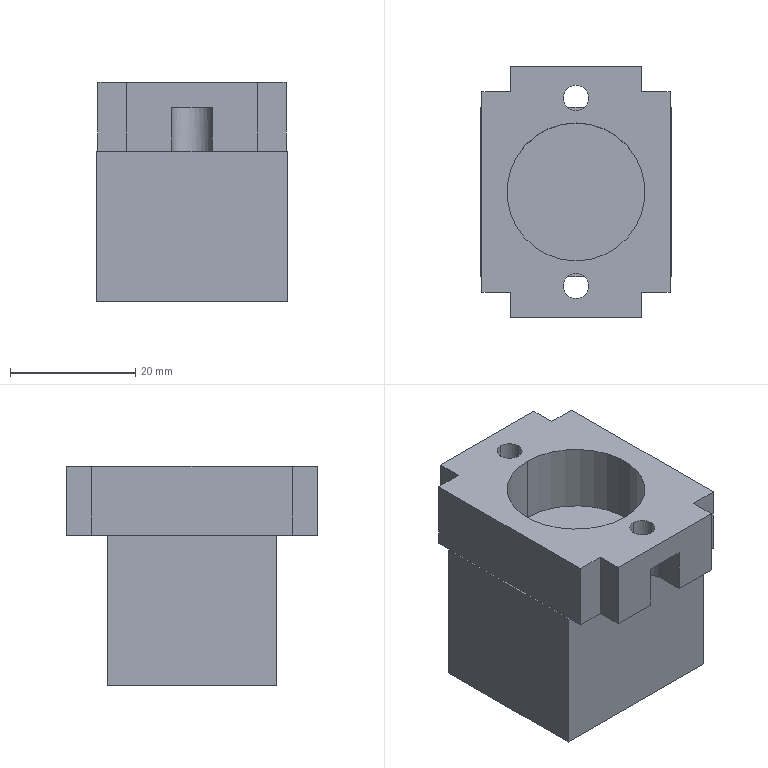Part | SolidWorks | features ImportedCurve 15, BaseBody 1 | 1 solid | 41 faces | box 30.5 x 40 x 35 mm | volume 27294 mm3 | plane 33 | cylinder 8 | commonest cylinder face diameters 4 x4 6.5 x2 22 x2
STEP:
#1=CARTESIAN_POINT('',(3.25,16.,0.));
#2=VERTEX_POINT('',#1);
#3=CARTESIAN_POINT('',(3.25,16.,7.));
#4=VERTEX_POINT('',#3);
#5=CARTESIAN_POINT('',(3.25,16.,0.));
#6=DIRECTION('',(0.,0.,1.));
#7=VECTOR('',#6,1000.);
#8=LINE('',#5,#7);
#9=EDGE_CURVE('',#2,#4,#8,.T.);
#10=ORIENTED_EDGE('',*,*,#9,.T.);
#11=CARTESIAN_POINT('',(3.25,20.,7.));
#12=VERTEX_POINT('',#11);
#13=CARTESIAN_POINT('',(3.25,20.,7.));
#14=DIRECTION('',(0.,-1.,0.));
#15=VECTOR('',#14,1000.);
#16=LINE('',#13,#15);
#17=EDGE_CURVE('',#12,#4,#16,.T.);
#18=ORIENTED_EDGE('',*,*,#17,.F.);
#19=CARTESIAN_POINT('',(3.25,20.,0.));
#20=VERTEX_POINT('',#19);
#21=CARTESIAN_POINT('',(3.25,20.,0.));
#22=DIRECTION('',(0.,0.,1.));
#23=VECTOR('',#22,1000.);
#24=LINE('',#21,#23);
#25=EDGE_CURVE('',#20,#12,#24,.T.);
#26=ORIENTED_EDGE('',*,*,#25,.F.);
#27=CARTESIAN_POINT('',(3.25,20.,0.));
#28=DIRECTION('',(0.,-1.,0.));
#29=VECTOR('',#28,1000.);
#30=LINE('',#27,#29);
#31=EDGE_CURVE('',#20,#2,#30,.T.);
#32=ORIENTED_EDGE('',*,*,#31,.T.);
#33=EDGE_LOOP('',(#10,#18,#26,#32));
#34=FACE_OUTER_BOUND('',#33,.T.);
#35=CARTESIAN_POINT('',(3.25,20.,0.));
#36=DIRECTION('',(1.,0.,0.));
#37=DIRECTION('',(0.,-1.,0.));
#38=AXIS2_PLACEMENT_3D('',#35,#36,#37);
#39=PLANE('',#38);
#40=ADVANCED_FACE('',(#34),#39,.F.);
#41=CARTESIAN_POINT('',(-15.25,13.5,0.));
#42=VERTEX_POINT('',#41);
#43=CARTESIAN_POINT('',(-15.25,13.5,-24.));
#44=VERTEX_POINT('',#43);
#45=CARTESIAN_POINT('',(-15.25,13.5,0.));
#46=DIRECTION('',(0.,0.,-1.));
#47=VECTOR('',#46,1000.);
#48=LINE('',#45,#47);
#49=EDGE_CURVE('',#42,#44,#48,.T.);
#50=ORIENTED_EDGE('',*,*,#49,.T.);
#51=CARTESIAN_POINT('',(-15.25,-13.5,-24.));
#52=VERTEX_POINT('',#51);
#53=CARTESIAN_POINT('',(-15.25,-13.5,-24.));
#54=DIRECTION('',(0.,1.,0.));
#55=VECTOR('',#54,1000.);
#56=LINE('',#53,#55);
#57=EDGE_CURVE('',#52,#44,#56,.T.);
#58=ORIENTED_EDGE('',*,*,#57,.F.);
#59=CARTESIAN_POINT('',(-15.25,-13.5,0.));
#60=VERTEX_POINT('',#59);
#61=CARTESIAN_POINT('',(-15.25,-13.5,0.));
#62=DIRECTION('',(0.,0.,-1.));
#63=VECTOR('',#62,1000.);
#64=LINE('',#61,#63);
#65=EDGE_CURVE('',#60,#52,#64,.T.);
#66=ORIENTED_EDGE('',*,*,#65,.F.);
#67=CARTESIAN_POINT('',(-15.25,-13.5,0.));
#68=DIRECTION('',(0.,1.,0.));
#69=VECTOR('',#68,1000.);
#70=LINE('',#67,#69);
#71=EDGE_CURVE('',#60,#42,#70,.T.);
#72=ORIENTED_EDGE('',*,*,#71,.T.);
#73=EDGE_LOOP('',(#50,#58,#66,#72));
#74=FACE_OUTER_BOUND('',#73,.T.);
#75=CARTESIAN_POINT('',(-15.25,-13.5,0.));
#76=DIRECTION('',(-1.,0.,0.));
#77=DIRECTION('',(0.,1.,0.));
#78=AXIS2_PLACEMENT_3D('',#75,#76,#77);
#79=PLANE('',#78);
#80=ADVANCED_FACE('',(#74),#79,.T.);
#81=CARTESIAN_POINT('',(15.25,13.5,-24.));
#82=VERTEX_POINT('',#81);
#83=CARTESIAN_POINT('',(-15.25,13.5,-24.));
#84=DIRECTION('',(1.,0.,0.));
#85=VECTOR('',#84,1000.);
#86=LINE('',#83,#85);
#87=EDGE_CURVE('',#44,#82,#86,.T.);
#88=ORIENTED_EDGE('',*,*,#87,.T.);
#89=CARTESIAN_POINT('',(15.25,-13.5,-24.));
#90=VERTEX_POINT('',#89);
#91=CARTESIAN_POINT('',(15.25,13.5,-24.));
#92=DIRECTION('',(0.,-1.,0.));
#93=VECTOR('',#92,1000.);
#94=LINE('',#91,#93);
#95=EDGE_CURVE('',#82,#90,#94,.T.);
#96=ORIENTED_EDGE('',*,*,#95,.T.);
#97=CARTESIAN_POINT('',(15.25,-13.5,-24.));
#98=DIRECTION('',(-1.,0.,0.));
#99=VECTOR('',#98,1000.);
#100=LINE('',#97,#99);
#101=EDGE_CURVE('',#90,#52,#100,.T.);
#102=ORIENTED_EDGE('',*,*,#101,.T.);
#103=ORIENTED_EDGE('',*,*,#57,.T.);
#104=EDGE_LOOP('',(#88,#96,#102,#103));
#105=FACE_OUTER_BOUND('',#104,.T.);
#106=CARTESIAN_POINT('',(0.,0.,-24.));
#107=DIRECTION('',(0.,0.,-1.));
#108=DIRECTION('',(1.,0.,0.));
#109=AXIS2_PLACEMENT_3D('',#106,#107,#108);
#110=PLANE('',#109);
#111=ADVANCED_FACE('',(#105),#110,.T.);
#112=CARTESIAN_POINT('',(15.25,-13.5,0.));
#113=VERTEX_POINT('',#112);
#114=CARTESIAN_POINT('',(15.25,-13.5,0.));
#115=DIRECTION('',(0.,0.,-1.));
#116=VECTOR('',#115,1000.);
#117=LINE('',#114,#116);
#118=EDGE_CURVE('',#113,#90,#117,.T.);
#119=ORIENTED_EDGE('',*,*,#118,.T.);
#120=ORIENTED_EDGE('',*,*,#95,.F.);
#121=CARTESIAN_POINT('',(15.25,13.5,0.));
#122=VERTEX_POINT('',#121);
#123=CARTESIAN_POINT('',(15.25,13.5,0.));
#124=DIRECTION('',(0.,0.,-1.));
#125=VECTOR('',#124,1000.);
#126=LINE('',#123,#125);
#127=EDGE_CURVE('',#122,#82,#126,.T.);
#128=ORIENTED_EDGE('',*,*,#127,.F.);
#129=CARTESIAN_POINT('',(15.25,13.5,0.));
#130=DIRECTION('',(0.,-1.,0.));
#131=VECTOR('',#130,1000.);
#132=LINE('',#129,#131);
#133=EDGE_CURVE('',#122,#113,#132,.T.);
#134=ORIENTED_EDGE('',*,*,#133,.T.);
#135=EDGE_LOOP('',(#119,#120,#128,#134));
#136=FACE_OUTER_BOUND('',#135,.T.);
#137=CARTESIAN_POINT('',(15.25,13.5,0.));
#138=DIRECTION('',(1.,0.,0.));
#139=DIRECTION('',(0.,-1.,0.));
#140=AXIS2_PLACEMENT_3D('',#137,#138,#139);
#141=PLANE('',#140);
#142=ADVANCED_FACE('',(#136),#141,.T.);
#143=ORIENTED_EDGE('',*,*,#133,.F.);
#144=CARTESIAN_POINT('',(15.,13.5,0.));
#145=VERTEX_POINT('',#144);
#146=CARTESIAN_POINT('',(15.,13.5,0.));
#147=DIRECTION('',(1.,0.,0.));
#148=VECTOR('',#147,1000.);
#149=LINE('',#146,#148);
#150=EDGE_CURVE('',#145,#122,#149,.T.);
#151=ORIENTED_EDGE('',*,*,#150,.F.);
#152=CARTESIAN_POINT('',(15.,-13.5,0.));
#153=VERTEX_POINT('',#152);
#154=CARTESIAN_POINT('',(15.,13.5,0.));
#155=DIRECTION('',(0.,-1.,0.));
#156=VECTOR('',#155,1000.);
#157=LINE('',#154,#156);
#158=EDGE_CURVE('',#145,#153,#157,.T.);
#159=ORIENTED_EDGE('',*,*,#158,.T.);
#160=CARTESIAN_POINT('',(15.25,-13.5,0.));
#161=DIRECTION('',(-1.,0.,0.));
#162=VECTOR('',#161,1000.);
#163=LINE('',#160,#162);
#164=EDGE_CURVE('',#113,#153,#163,.T.);
#165=ORIENTED_EDGE('',*,*,#164,.F.);
#166=EDGE_LOOP('',(#143,#151,#159,#165));
#167=FACE_OUTER_BOUND('',#166,.T.);
#168=CARTESIAN_POINT('',(0.,0.,0.));
#169=DIRECTION('',(0.,0.,-1.));
#170=DIRECTION('',(1.,0.,0.));
#171=AXIS2_PLACEMENT_3D('',#168,#169,#170);
#172=PLANE('',#171);
#173=ADVANCED_FACE('',(#167),#172,.F.);
#174=CARTESIAN_POINT('',(0.,-11.,11.));
#175=VERTEX_POINT('',#174);
#176=CARTESIAN_POINT('',(0.,-11.,0.));
#177=VERTEX_POINT('',#176);
#178=CARTESIAN_POINT('',(0.,-11.,11.));
#179=DIRECTION('',(0.,0.,-1.));
#180=VECTOR('',#179,1000.);
#181=LINE('',#178,#180);
#182=EDGE_CURVE('',#175,#177,#181,.T.);
#183=ORIENTED_EDGE('',*,*,#182,.F.);
#184=CARTESIAN_POINT('',(0.,11.,11.));
#185=VERTEX_POINT('',#184);
#186=CARTESIAN_POINT('',(0.,0.,11.));
#187=DIRECTION('',(0.,0.,1.));
#188=DIRECTION('',(0.,-1.,0.));
#189=AXIS2_PLACEMENT_3D('',#186,#187,#188);
#190=CIRCLE('',#189,11.);
#191=EDGE_CURVE('',#175,#185,#190,.T.);
#192=ORIENTED_EDGE('',*,*,#191,.T.);
#193=CARTESIAN_POINT('',(0.,11.,0.));
#194=VERTEX_POINT('',#193);
#195=CARTESIAN_POINT('',(0.,11.,11.));
#196=DIRECTION('',(0.,0.,-1.));
#197=VECTOR('',#196,1000.);
#198=LINE('',#195,#197);
#199=EDGE_CURVE('',#185,#194,#198,.T.);
#200=ORIENTED_EDGE('',*,*,#199,.T.);
#201=CARTESIAN_POINT('',(0.,0.,0.));
#202=DIRECTION('',(0.,0.,1.));
#203=DIRECTION('',(0.,-1.,0.));
#204=AXIS2_PLACEMENT_3D('',#201,#202,#203);
#205=CIRCLE('',#204,11.);
#206=EDGE_CURVE('',#177,#194,#205,.T.);
#207=ORIENTED_EDGE('',*,*,#206,.F.);
#208=EDGE_LOOP('',(#183,#192,#200,#207));
#209=FACE_OUTER_BOUND('',#208,.T.);
#210=CARTESIAN_POINT('',(0.,0.,11.));
#211=DIRECTION('',(0.,0.,1.));
#212=DIRECTION('',(0.,1.,0.));
#213=AXIS2_PLACEMENT_3D('',#210,#211,#212);
#214=CYLINDRICAL_SURFACE('',#213,11.);
#215=ADVANCED_FACE('',(#209),#214,.F.);
#216=ORIENTED_EDGE('',*,*,#206,.T.);
#217=CARTESIAN_POINT('',(0.,0.,0.));
#218=DIRECTION('',(0.,0.,1.));
#219=DIRECTION('',(0.,1.,0.));
#220=AXIS2_PLACEMENT_3D('',#217,#218,#219);
#221=CIRCLE('',#220,11.);
#222=EDGE_CURVE('',#194,#177,#221,.T.);
#223=ORIENTED_EDGE('',*,*,#222,.T.);
#224=EDGE_LOOP('',(#216,#223));
#225=FACE_OUTER_BOUND('',#224,.T.);
#226=CARTESIAN_POINT('',(0.,0.,0.));
#227=DIRECTION('',(0.,0.,-1.));
#228=DIRECTION('',(1.,0.,0.));
#229=AXIS2_PLACEMENT_3D('',#226,#227,#228);
#230=PLANE('',#229);
#231=ADVANCED_FACE('',(#225),#230,.F.);
#232=ORIENTED_EDGE('',*,*,#199,.F.);
#233=CARTESIAN_POINT('',(0.,0.,11.));
#234=DIRECTION('',(0.,0.,1.));
#235=DIRECTION('',(0.,1.,0.));
#236=AXIS2_PLACEMENT_3D('',#233,#234,#235);
#237=CIRCLE('',#236,11.);
#238=EDGE_CURVE('',#185,#175,#237,.T.);
#239=ORIENTED_EDGE('',*,*,#238,.T.);
#240=ORIENTED_EDGE('',*,*,#182,.T.);
#241=ORIENTED_EDGE('',*,*,#222,.F.);
#242=EDGE_LOOP('',(#232,#239,#240,#241));
#243=FACE_OUTER_BOUND('',#242,.T.);
#244=CARTESIAN_POINT('',(0.,0.,11.));
#245=DIRECTION('',(0.,0.,1.));
#246=DIRECTION('',(0.,1.,0.));
#247=AXIS2_PLACEMENT_3D('',#244,#245,#246);
#248=CYLINDRICAL_SURFACE('',#247,11.);
#249=ADVANCED_FACE('',(#243),#248,.F.);
#250=CARTESIAN_POINT('',(0.,17.,11.));
#251=VERTEX_POINT('',#250);
#252=CARTESIAN_POINT('',(0.,17.,7.));
#253=VERTEX_POINT('',#252);
#254=CARTESIAN_POINT('',(0.,17.,11.));
#255=DIRECTION('',(0.,0.,-1.));
#256=VECTOR('',#255,1000.);
#257=LINE('',#254,#256);
#258=EDGE_CURVE('',#251,#253,#257,.T.);
#259=ORIENTED_EDGE('',*,*,#258,.T.);
#260=CARTESIAN_POINT('',(0.,13.,7.));
#261=VERTEX_POINT('',#260);
#262=CARTESIAN_POINT('',(0.,15.,7.));
#263=DIRECTION('',(0.,0.,1.));
#264=DIRECTION('',(0.,-1.,0.));
#265=AXIS2_PLACEMENT_3D('',#262,#263,#264);
#266=CIRCLE('',#265,2.);
#267=EDGE_CURVE('',#261,#253,#266,.T.);
#268=ORIENTED_EDGE('',*,*,#267,.F.);
#269=CARTESIAN_POINT('',(0.,13.,11.));
#270=VERTEX_POINT('',#269);
#271=CARTESIAN_POINT('',(0.,13.,11.));
#272=DIRECTION('',(0.,0.,-1.));
#273=VECTOR('',#272,1000.);
#274=LINE('',#271,#273);
#275=EDGE_CURVE('',#270,#261,#274,.T.);
#276=ORIENTED_EDGE('',*,*,#275,.F.);
#277=CARTESIAN_POINT('',(0.,15.,11.));
#278=DIRECTION('',(0.,0.,1.));
#279=DIRECTION('',(0.,-1.,0.));
#280=AXIS2_PLACEMENT_3D('',#277,#278,#279);
#281=CIRCLE('',#280,2.);
#282=EDGE_CURVE('',#270,#251,#281,.T.);
#283=ORIENTED_EDGE('',*,*,#282,.T.);
#284=EDGE_LOOP('',(#259,#268,#276,#283));
#285=FACE_OUTER_BOUND('',#284,.T.);
#286=CARTESIAN_POINT('',(0.,15.,11.));
#287=DIRECTION('',(0.,0.,1.));
#288=DIRECTION('',(0.,1.,0.));
#289=AXIS2_PLACEMENT_3D('',#286,#287,#288);
#290=CYLINDRICAL_SURFACE('',#289,2.);
#291=ADVANCED_FACE('',(#285),#290,.F.);
#292=ORIENTED_EDGE('',*,*,#275,.T.);
#293=CARTESIAN_POINT('',(0.,15.,7.));
#294=DIRECTION('',(0.,0.,1.));
#295=DIRECTION('',(0.,1.,0.));
#296=AXIS2_PLACEMENT_3D('',#293,#294,#295);
#297=CIRCLE('',#296,2.);
#298=EDGE_CURVE('',#253,#261,#297,.T.);
#299=ORIENTED_EDGE('',*,*,#298,.F.);
#300=ORIENTED_EDGE('',*,*,#258,.F.);
#301=CARTESIAN_POINT('',(0.,15.,11.));
#302=DIRECTION('',(0.,0.,1.));
#303=DIRECTION('',(0.,1.,0.));
#304=AXIS2_PLACEMENT_3D('',#301,#302,#303);
#305=CIRCLE('',#304,2.);
#306=EDGE_CURVE('',#251,#270,#305,.T.);
#307=ORIENTED_EDGE('',*,*,#306,.T.);
#308=EDGE_LOOP('',(#292,#299,#300,#307));
#309=FACE_OUTER_BOUND('',#308,.T.);
#310=CARTESIAN_POINT('',(0.,15.,11.));
#311=DIRECTION('',(0.,0.,1.));
#312=DIRECTION('',(0.,1.,0.));
#313=AXIS2_PLACEMENT_3D('',#310,#311,#312);
#314=CYLINDRICAL_SURFACE('',#313,2.);
#315=ADVANCED_FACE('',(#309),#314,.F.);
#316=CARTESIAN_POINT('',(-10.5,-20.,0.));
#317=VERTEX_POINT('',#316);
#318=CARTESIAN_POINT('',(-10.5,-20.,11.));
#319=VERTEX_POINT('',#318);
#320=CARTESIAN_POINT('',(-10.5,-20.,0.));
#321=DIRECTION('',(0.,0.,1.));
#322=VECTOR('',#321,1000.);
#323=LINE('',#320,#322);
#324=EDGE_CURVE('',#317,#319,#323,.T.);
#325=ORIENTED_EDGE('',*,*,#324,.T.);
#326=CARTESIAN_POINT('',(-10.5,-16.,11.));
#327=VERTEX_POINT('',#326);
#328=CARTESIAN_POINT('',(-10.5,-16.,11.));
#329=DIRECTION('',(0.,-1.,0.));
#330=VECTOR('',#329,1000.);
#331=LINE('',#328,#330);
#332=EDGE_CURVE('',#327,#319,#331,.T.);
#333=ORIENTED_EDGE('',*,*,#332,.F.);
#334=CARTESIAN_POINT('',(-10.5,-16.,0.));
#335=VERTEX_POINT('',#334);
#336=CARTESIAN_POINT('',(-10.5,-16.,0.));
#337=DIRECTION('',(0.,0.,1.));
#338=VECTOR('',#337,1000.);
#339=LINE('',#336,#338);
#340=EDGE_CURVE('',#335,#327,#339,.T.);
#341=ORIENTED_EDGE('',*,*,#340,.F.);
#342=CARTESIAN_POINT('',(-10.5,-16.,0.));
#343=DIRECTION('',(0.,-1.,0.));
#344=VECTOR('',#343,1000.);
#345=LINE('',#342,#344);
#346=EDGE_CURVE('',#335,#317,#345,.T.);
#347=ORIENTED_EDGE('',*,*,#346,.T.);
#348=EDGE_LOOP('',(#325,#333,#341,#347));
#349=FACE_OUTER_BOUND('',#348,.T.);
#350=CARTESIAN_POINT('',(-10.5,-16.,0.));
#351=DIRECTION('',(-1.,0.,0.));
#352=DIRECTION('',(0.,-1.,0.));
#353=AXIS2_PLACEMENT_3D('',#350,#351,#352);
#354=PLANE('',#353);
#355=ADVANCED_FACE('',(#349),#354,.T.);
#356=CARTESIAN_POINT('',(0.,-13.,11.));
#357=VERTEX_POINT('',#356);
#358=CARTESIAN_POINT('',(0.,-13.,7.));
#359=VERTEX_POINT('',#358);
#360=CARTESIAN_POINT('',(0.,-13.,11.));
#361=DIRECTION('',(0.,0.,-1.));
#362=VECTOR('',#361,1000.);
#363=LINE('',#360,#362);
#364=EDGE_CURVE('',#357,#359,#363,.T.);
#365=ORIENTED_EDGE('',*,*,#364,.T.);
#366=CARTESIAN_POINT('',(0.,-17.,7.));
#367=VERTEX_POINT('',#366);
#368=CARTESIAN_POINT('',(0.,-15.,7.));
#369=DIRECTION('',(0.,0.,1.));
#370=DIRECTION('',(0.,-1.,0.));
#371=AXIS2_PLACEMENT_3D('',#368,#369,#370);
#372=CIRCLE('',#371,2.);
#373=EDGE_CURVE('',#367,#359,#372,.T.);
#374=ORIENTED_EDGE('',*,*,#373,.F.);
#375=CARTESIAN_POINT('',(0.,-17.,11.));
#376=VERTEX_POINT('',#375);
#377=CARTESIAN_POINT('',(0.,-17.,11.));
#378=DIRECTION('',(0.,0.,-1.));
#379=VECTOR('',#378,1000.);
#380=LINE('',#377,#379);
#381=EDGE_CURVE('',#376,#367,#380,.T.);
#382=ORIENTED_EDGE('',*,*,#381,.F.);
#383=CARTESIAN_POINT('',(0.,-15.,11.));
#384=DIRECTION('',(0.,0.,1.));
#385=DIRECTION('',(0.,-1.,0.));
#386=AXIS2_PLACEMENT_3D('',#383,#384,#385);
#387=CIRCLE('',#386,2.);
#388=EDGE_CURVE('',#376,#357,#387,.T.);
#389=ORIENTED_EDGE('',*,*,#388,.T.);
#390=EDGE_LOOP('',(#365,#374,#382,#389));
#391=FACE_OUTER_BOUND('',#390,.T.);
#392=CARTESIAN_POINT('',(0.,-15.,11.));
#393=DIRECTION('',(0.,0.,1.));
#394=DIRECTION('',(0.,1.,0.));
#395=AXIS2_PLACEMENT_3D('',#392,#393,#394);
#396=CYLINDRICAL_SURFACE('',#395,2.);
#397=ADVANCED_FACE('',(#391),#396,.F.);
#398=ORIENTED_EDGE('',*,*,#381,.T.);
#399=CARTESIAN_POINT('',(0.,-15.,7.));
#400=DIRECTION('',(0.,0.,1.));
#401=DIRECTION('',(0.,1.,0.));
#402=AXIS2_PLACEMENT_3D('',#399,#400,#401);
#403=CIRCLE('',#402,2.);
#404=EDGE_CURVE('',#359,#367,#403,.T.);
#405=ORIENTED_EDGE('',*,*,#404,.F.);
#406=ORIENTED_EDGE('',*,*,#364,.F.);
#407=CARTESIAN_POINT('',(0.,-15.,11.));
#408=DIRECTION('',(0.,0.,1.));
#409=DIRECTION('',(0.,1.,0.));
#410=AXIS2_PLACEMENT_3D('',#407,#408,#409);
#411=CIRCLE('',#410,2.);
#412=EDGE_CURVE('',#357,#376,#411,.T.);
#413=ORIENTED_EDGE('',*,*,#412,.T.);
#414=EDGE_LOOP('',(#398,#405,#406,#413));
#415=FACE_OUTER_BOUND('',#414,.T.);
#416=CARTESIAN_POINT('',(0.,-15.,11.));
#417=DIRECTION('',(0.,0.,1.));
#418=DIRECTION('',(0.,1.,0.));
#419=AXIS2_PLACEMENT_3D('',#416,#417,#418);
#420=CYLINDRICAL_SURFACE('',#419,2.);
#421=ADVANCED_FACE('',(#415),#420,.F.);
#422=CARTESIAN_POINT('',(-3.25,-16.,0.));
#423=VERTEX_POINT('',#422);
#424=CARTESIAN_POINT('',(-3.25,-16.,7.));
#425=VERTEX_POINT('',#424);
#426=CARTESIAN_POINT('',(-3.25,-16.,0.));
#427=DIRECTION('',(0.,0.,1.));
#428=VECTOR('',#427,1000.);
#429=LINE('',#426,#428);
#430=EDGE_CURVE('',#423,#425,#429,.T.);
#431=ORIENTED_EDGE('',*,*,#430,.T.);
#432=CARTESIAN_POINT('',(-3.25,-20.,7.));
#433=VERTEX_POINT('',#432);
#434=CARTESIAN_POINT('',(-3.25,-20.,7.));
#435=DIRECTION('',(0.,1.,0.));
#436=VECTOR('',#435,1000.);
#437=LINE('',#434,#436);
#438=EDGE_CURVE('',#433,#425,#437,.T.);
#439=ORIENTED_EDGE('',*,*,#438,.F.);
#440=CARTESIAN_POINT('',(-3.25,-20.,0.));
#441=VERTEX_POINT('',#440);
#442=CARTESIAN_POINT('',(-3.25,-20.,0.));
#443=DIRECTION('',(0.,0.,1.));
#444=VECTOR('',#443,1000.);
#445=LINE('',#442,#444);
#446=EDGE_CURVE('',#441,#433,#445,.T.);
#447=ORIENTED_EDGE('',*,*,#446,.F.);
#448=CARTESIAN_POINT('',(-3.25,-20.,0.));
#449=DIRECTION('',(0.,1.,0.));
#450=VECTOR('',#449,1000.);
#451=LINE('',#448,#450);
#452=EDGE_CURVE('',#441,#423,#451,.T.);
#453=ORIENTED_EDGE('',*,*,#452,.T.);
#454=EDGE_LOOP('',(#431,#439,#447,#453));
#455=FACE_OUTER_BOUND('',#454,.T.);
#456=CARTESIAN_POINT('',(-3.25,-20.,0.));
#457=DIRECTION('',(-1.,0.,0.));
#458=DIRECTION('',(0.,1.,0.));
#459=AXIS2_PLACEMENT_3D('',#456,#457,#458);
#460=PLANE('',#459);
#461=ADVANCED_FACE('',(#455),#460,.F.);
#462=CARTESIAN_POINT('',(2.077,-13.5,0.));
#463=VERTEX_POINT('',#462);
#464=CARTESIAN_POINT('',(-2.077,-13.5,0.));
#465=VERTEX_POINT('',#464);
#466=CARTESIAN_POINT('',(2.077,-13.5,0.));
#467=DIRECTION('',(-1.,0.,0.));
#468=VECTOR('',#467,1000.);
#469=LINE('',#466,#468);
#470=EDGE_CURVE('',#463,#465,#469,.T.);
#471=ORIENTED_EDGE('',*,*,#470,.F.);
#472=CARTESIAN_POINT('',(0.,-16.,0.));
#473=DIRECTION('',(0.,0.,-1.));
#474=DIRECTION('',(-0.639,0.7692,0.));
#475=AXIS2_PLACEMENT_3D('',#472,#473,#474);
#476=CIRCLE('',#475,3.25);
#477=EDGE_CURVE('',#465,#463,#476,.T.);
#478=ORIENTED_EDGE('',*,*,#477,.F.);
#479=EDGE_LOOP('',(#471,#478));
#480=FACE_OUTER_BOUND('',#479,.T.);
#481=CARTESIAN_POINT('',(0.,0.,0.));
#482=DIRECTION('',(0.,0.,-1.));
#483=DIRECTION('',(1.,0.,0.));
#484=AXIS2_PLACEMENT_3D('',#481,#482,#483);
#485=PLANE('',#484);
#486=ADVANCED_FACE('',(#480),#485,.F.);
#487=CARTESIAN_POINT('',(3.25,-16.,0.));
#488=VERTEX_POINT('',#487);
#489=CARTESIAN_POINT('',(0.,-16.,0.));
#490=DIRECTION('',(0.,0.,-1.));
#491=DIRECTION('',(0.639,0.7692,0.));
#492=AXIS2_PLACEMENT_3D('',#489,#490,#491);
#493=CIRCLE('',#492,3.25);
#494=EDGE_CURVE('',#463,#488,#493,.T.);
#495=ORIENTED_EDGE('',*,*,#494,.T.);
#496=CARTESIAN_POINT('',(3.25,-16.,7.));
#497=VERTEX_POINT('',#496);
#498=CARTESIAN_POINT('',(3.25,-16.,0.));
#499=DIRECTION('',(0.,0.,1.));
#500=VECTOR('',#499,1000.);
#501=LINE('',#498,#500);
#502=EDGE_CURVE('',#488,#497,#501,.T.);
#503=ORIENTED_EDGE('',*,*,#502,.T.);
#504=CARTESIAN_POINT('',(0.,-16.,7.));
#505=DIRECTION('',(0.,0.,-1.));
#506=DIRECTION('',(-1.,0.,0.));
#507=AXIS2_PLACEMENT_3D('',#504,#505,#506);
#508=CIRCLE('',#507,3.25);
#509=EDGE_CURVE('',#425,#497,#508,.T.);
#510=ORIENTED_EDGE('',*,*,#509,.F.);
#511=ORIENTED_EDGE('',*,*,#430,.F.);
#512=CARTESIAN_POINT('',(0.,-16.,0.));
#513=DIRECTION('',(0.,0.,-1.));
#514=DIRECTION('',(-1.,0.,0.));
#515=AXIS2_PLACEMENT_3D('',#512,#513,#514);
#516=CIRCLE('',#515,3.25);
#517=EDGE_CURVE('',#423,#465,#516,.T.);
#518=ORIENTED_EDGE('',*,*,#517,.T.);
#519=ORIENTED_EDGE('',*,*,#477,.T.);
#520=EDGE_LOOP('',(#495,#503,#510,#511,#518,#519));
#521=FACE_OUTER_BOUND('',#520,.T.);
#522=CARTESIAN_POINT('',(0.,-16.,0.));
#523=DIRECTION('',(0.,0.,-1.));
#524=DIRECTION('',(1.,0.,0.));
#525=AXIS2_PLACEMENT_3D('',#522,#523,#524);
#526=CYLINDRICAL_SURFACE('',#525,3.25);
#527=ADVANCED_FACE('',(#521),#526,.F.);
#528=CARTESIAN_POINT('',(3.25,-20.,0.));
#529=VERTEX_POINT('',#528);
#530=CARTESIAN_POINT('',(3.25,-20.,7.));
#531=VERTEX_POINT('',#530);
#532=CARTESIAN_POINT('',(3.25,-20.,0.));
#533=DIRECTION('',(0.,0.,1.));
#534=VECTOR('',#533,1000.);
#535=LINE('',#532,#534);
#536=EDGE_CURVE('',#529,#531,#535,.T.);
#537=ORIENTED_EDGE('',*,*,#536,.T.);
#538=CARTESIAN_POINT('',(3.25,-16.,7.));
#539=DIRECTION('',(0.,-1.,0.));
#540=VECTOR('',#539,1000.);
#541=LINE('',#538,#540);
#542=EDGE_CURVE('',#497,#531,#541,.T.);
#543=ORIENTED_EDGE('',*,*,#542,.F.);
#544=ORIENTED_EDGE('',*,*,#502,.F.);
#545=CARTESIAN_POINT('',(3.25,-20.,0.));
#546=DIRECTION('',(0.,1.,0.));
#547=VECTOR('',#546,1000.);
#548=LINE('',#545,#547);
#549=EDGE_CURVE('',#529,#488,#548,.T.);
#550=ORIENTED_EDGE('',*,*,#549,.F.);
#551=EDGE_LOOP('',(#537,#543,#544,#550));
#552=FACE_OUTER_BOUND('',#551,.T.);
#553=CARTESIAN_POINT('',(3.25,-16.,0.));
#554=DIRECTION('',(1.,0.,0.));
#555=DIRECTION('',(0.,-1.,0.));
#556=AXIS2_PLACEMENT_3D('',#553,#554,#555);
#557=PLANE('',#556);
#558=ADVANCED_FACE('',(#552),#557,.F.);
#559=ORIENTED_EDGE('',*,*,#373,.T.);
#560=ORIENTED_EDGE('',*,*,#404,.T.);
#561=EDGE_LOOP('',(#559,#560));
#562=FACE_BOUND('',#561,.T.);
#563=ORIENTED_EDGE('',*,*,#438,.T.);
#564=ORIENTED_EDGE('',*,*,#509,.T.);
#565=ORIENTED_EDGE('',*,*,#542,.T.);
#566=CARTESIAN_POINT('',(-3.25,-20.,7.));
#567=DIRECTION('',(1.,0.,0.));
#568=VECTOR('',#567,1000.);
#569=LINE('',#566,#568);
#570=EDGE_CURVE('',#433,#531,#569,.T.);
#571=ORIENTED_EDGE('',*,*,#570,.F.);
#572=EDGE_LOOP('',(#563,#564,#565,#571));
#573=FACE_OUTER_BOUND('',#572,.T.);
#574=CARTESIAN_POINT('',(0.,0.,7.));
#575=DIRECTION('',(0.,0.,-1.));
#576=DIRECTION('',(1.,0.,0.));
#577=AXIS2_PLACEMENT_3D('',#574,#575,#576);
#578=PLANE('',#577);
#579=ADVANCED_FACE('',(#562,#573),#578,.T.);
#580=ORIENTED_EDGE('',*,*,#536,.F.);
#581=CARTESIAN_POINT('',(10.5,-20.,0.));
#582=VERTEX_POINT('',#581);
#583=CARTESIAN_POINT('',(3.25,-20.,0.));
#584=DIRECTION('',(1.,0.,0.));
#585=VECTOR('',#584,1000.);
#586=LINE('',#583,#585);
#587=EDGE_CURVE('',#529,#582,#586,.T.);
#588=ORIENTED_EDGE('',*,*,#587,.T.);
#589=CARTESIAN_POINT('',(10.5,-20.,11.));
#590=VERTEX_POINT('',#589);
#591=CARTESIAN_POINT('',(10.5,-20.,0.));
#592=DIRECTION('',(0.,0.,1.));
#593=VECTOR('',#592,1000.);
#594=LINE('',#591,#593);
#595=EDGE_CURVE('',#582,#590,#594,.T.);
#596=ORIENTED_EDGE('',*,*,#595,.T.);
#597=CARTESIAN_POINT('',(-10.5,-20.,11.));
#598=DIRECTION('',(1.,0.,0.));
#599=VECTOR('',#598,1000.);
#600=LINE('',#597,#599);
#601=EDGE_CURVE('',#319,#590,#600,.T.);
#602=ORIENTED_EDGE('',*,*,#601,.F.);
#603=ORIENTED_EDGE('',*,*,#324,.F.);
#604=CARTESIAN_POINT('',(-10.5,-20.,0.));
#605=DIRECTION('',(1.,0.,0.));
#606=VECTOR('',#605,1000.);
#607=LINE('',#604,#606);
#608=EDGE_CURVE('',#317,#441,#607,.T.);
#609=ORIENTED_EDGE('',*,*,#608,.T.);
#610=ORIENTED_EDGE('',*,*,#446,.T.);
#611=ORIENTED_EDGE('',*,*,#570,.T.);
#612=EDGE_LOOP('',(#580,#588,#596,#602,#603,#609,#610,#611));
#613=FACE_OUTER_BOUND('',#612,.T.);
#614=CARTESIAN_POINT('',(-10.5,-20.,0.));
#615=DIRECTION('',(0.,-1.,0.));
#616=DIRECTION('',(1.,0.,0.));
#617=AXIS2_PLACEMENT_3D('',#614,#615,#616);
#618=PLANE('',#617);
#619=ADVANCED_FACE('',(#613),#618,.T.);
#620=CARTESIAN_POINT('',(10.5,-16.,0.));
#621=VERTEX_POINT('',#620);
#622=CARTESIAN_POINT('',(10.5,-16.,11.));
#623=VERTEX_POINT('',#622);
#624=CARTESIAN_POINT('',(10.5,-16.,0.));
#625=DIRECTION('',(0.,0.,1.));
#626=VECTOR('',#625,1000.);
#627=LINE('',#624,#626);
#628=EDGE_CURVE('',#621,#623,#627,.T.);
#629=ORIENTED_EDGE('',*,*,#628,.T.);
#630=CARTESIAN_POINT('',(10.5,-20.,11.));
#631=DIRECTION('',(0.,1.,0.));
#632=VECTOR('',#631,1000.);
#633=LINE('',#630,#632);
#634=EDGE_CURVE('',#590,#623,#633,.T.);
#635=ORIENTED_EDGE('',*,*,#634,.F.);
#636=ORIENTED_EDGE('',*,*,#595,.F.);
#637=CARTESIAN_POINT('',(10.5,-20.,0.));
#638=DIRECTION('',(0.,1.,0.));
#639=VECTOR('',#638,1000.);
#640=LINE('',#637,#639);
#641=EDGE_CURVE('',#582,#621,#640,.T.);
#642=ORIENTED_EDGE('',*,*,#641,.T.);
#643=EDGE_LOOP('',(#629,#635,#636,#642));
#644=FACE_OUTER_BOUND('',#643,.T.);
#645=CARTESIAN_POINT('',(10.5,-20.,0.));
#646=DIRECTION('',(1.,0.,0.));
#647=DIRECTION('',(0.,1.,0.));
#648=AXIS2_PLACEMENT_3D('',#645,#646,#647);
#649=PLANE('',#648);
#650=ADVANCED_FACE('',(#644),#649,.T.);
#651=CARTESIAN_POINT('',(15.,-16.,0.));
#652=VERTEX_POINT('',#651);
#653=CARTESIAN_POINT('',(15.,-16.,11.));
#654=VERTEX_POINT('',#653);
#655=CARTESIAN_POINT('',(15.,-16.,0.));
#656=DIRECTION('',(0.,0.,1.));
#657=VECTOR('',#656,1000.);
#658=LINE('',#655,#657);
#659=EDGE_CURVE('',#652,#654,#658,.T.);
#660=ORIENTED_EDGE('',*,*,#659,.T.);
#661=CARTESIAN_POINT('',(10.5,-16.,11.));
#662=DIRECTION('',(1.,0.,0.));
#663=VECTOR('',#662,1000.);
#664=LINE('',#661,#663);
#665=EDGE_CURVE('',#623,#654,#664,.T.);
#666=ORIENTED_EDGE('',*,*,#665,.F.);
#667=ORIENTED_EDGE('',*,*,#628,.F.);
#668=CARTESIAN_POINT('',(10.5,-16.,0.));
#669=DIRECTION('',(1.,0.,0.));
#670=VECTOR('',#669,1000.);
#671=LINE('',#668,#670);
#672=EDGE_CURVE('',#621,#652,#671,.T.);
#673=ORIENTED_EDGE('',*,*,#672,.T.);
#674=EDGE_LOOP('',(#660,#666,#667,#673));
#675=FACE_OUTER_BOUND('',#674,.T.);
#676=CARTESIAN_POINT('',(10.5,-16.,0.));
#677=DIRECTION('',(0.,-1.,0.));
#678=DIRECTION('',(1.,0.,0.));
#679=AXIS2_PLACEMENT_3D('',#676,#677,#678);
#680=PLANE('',#679);
#681=ADVANCED_FACE('',(#675),#680,.T.);
#682=CARTESIAN_POINT('',(10.5,16.,0.));
#683=VERTEX_POINT('',#682);
#684=CARTESIAN_POINT('',(10.5,16.,11.));
#685=VERTEX_POINT('',#684);
#686=CARTESIAN_POINT('',(10.5,16.,0.));
#687=DIRECTION('',(0.,0.,1.));
#688=VECTOR('',#687,1000.);
#689=LINE('',#686,#688);
#690=EDGE_CURVE('',#683,#685,#689,.T.);
#691=ORIENTED_EDGE('',*,*,#690,.T.);
#692=CARTESIAN_POINT('',(15.,16.,11.));
#693=VERTEX_POINT('',#692);
#694=CARTESIAN_POINT('',(15.,16.,11.));
#695=DIRECTION('',(-1.,0.,0.));
#696=VECTOR('',#695,1000.);
#697=LINE('',#694,#696);
#698=EDGE_CURVE('',#693,#685,#697,.T.);
#699=ORIENTED_EDGE('',*,*,#698,.F.);
#700=CARTESIAN_POINT('',(15.,16.,0.));
#701=VERTEX_POINT('',#700);
#702=CARTESIAN_POINT('',(15.,16.,0.));
#703=DIRECTION('',(0.,0.,1.));
#704=VECTOR('',#703,1000.);
#705=LINE('',#702,#704);
#706=EDGE_CURVE('',#701,#693,#705,.T.);
#707=ORIENTED_EDGE('',*,*,#706,.F.);
#708=CARTESIAN_POINT('',(15.,16.,0.));
#709=DIRECTION('',(-1.,0.,0.));
#710=VECTOR('',#709,1000.);
#711=LINE('',#708,#710);
#712=EDGE_CURVE('',#701,#683,#711,.T.);
#713=ORIENTED_EDGE('',*,*,#712,.T.);
#714=EDGE_LOOP('',(#691,#699,#707,#713));
#715=FACE_OUTER_BOUND('',#714,.T.);
#716=CARTESIAN_POINT('',(15.,16.,0.));
#717=DIRECTION('',(0.,1.,0.));
#718=DIRECTION('',(-1.,0.,0.));
#719=AXIS2_PLACEMENT_3D('',#716,#717,#718);
#720=PLANE('',#719);
#721=ADVANCED_FACE('',(#715),#720,.T.);
#722=CARTESIAN_POINT('',(10.5,20.,0.));
#723=VERTEX_POINT('',#722);
#724=CARTESIAN_POINT('',(10.5,20.,11.));
#725=VERTEX_POINT('',#724);
#726=CARTESIAN_POINT('',(10.5,20.,0.));
#727=DIRECTION('',(0.,0.,1.));
#728=VECTOR('',#727,1000.);
#729=LINE('',#726,#728);
#730=EDGE_CURVE('',#723,#725,#729,.T.);
#731=ORIENTED_EDGE('',*,*,#730,.T.);
#732=CARTESIAN_POINT('',(10.5,16.,11.));
#733=DIRECTION('',(0.,1.,0.));
#734=VECTOR('',#733,1000.);
#735=LINE('',#732,#734);
#736=EDGE_CURVE('',#685,#725,#735,.T.);
#737=ORIENTED_EDGE('',*,*,#736,.F.);
#738=ORIENTED_EDGE('',*,*,#690,.F.);
#739=CARTESIAN_POINT('',(10.5,16.,0.));
#740=DIRECTION('',(0.,1.,0.));
#741=VECTOR('',#740,1000.);
#742=LINE('',#739,#741);
#743=EDGE_CURVE('',#683,#723,#742,.T.);
#744=ORIENTED_EDGE('',*,*,#743,.T.);
#745=EDGE_LOOP('',(#731,#737,#738,#744));
#746=FACE_OUTER_BOUND('',#745,.T.);
#747=CARTESIAN_POINT('',(10.5,16.,0.));
#748=DIRECTION('',(1.,0.,0.));
#749=DIRECTION('',(0.,1.,0.));
#750=AXIS2_PLACEMENT_3D('',#747,#748,#749);
#751=PLANE('',#750);
#752=ADVANCED_FACE('',(#746),#751,.T.);
#753=ORIENTED_EDGE('',*,*,#191,.F.);
#754=ORIENTED_EDGE('',*,*,#238,.F.);
#755=EDGE_LOOP('',(#753,#754));
#756=FACE_BOUND('',#755,.T.);
#757=ORIENTED_EDGE('',*,*,#388,.F.);
#758=ORIENTED_EDGE('',*,*,#412,.F.);
#759=EDGE_LOOP('',(#757,#758));
#760=FACE_BOUND('',#759,.T.);
#761=ORIENTED_EDGE('',*,*,#282,.F.);
#762=ORIENTED_EDGE('',*,*,#306,.F.);
#763=EDGE_LOOP('',(#761,#762));
#764=FACE_BOUND('',#763,.T.);
#765=CARTESIAN_POINT('',(-15.,-16.,11.));
#766=VERTEX_POINT('',#765);
#767=CARTESIAN_POINT('',(-15.,-16.,11.));
#768=DIRECTION('',(1.,0.,0.));
#769=VECTOR('',#768,1000.);
#770=LINE('',#767,#769);
#771=EDGE_CURVE('',#766,#327,#770,.T.);
#772=ORIENTED_EDGE('',*,*,#771,.T.);
#773=ORIENTED_EDGE('',*,*,#332,.T.);
#774=ORIENTED_EDGE('',*,*,#601,.T.);
#775=ORIENTED_EDGE('',*,*,#634,.T.);
#776=ORIENTED_EDGE('',*,*,#665,.T.);
#777=CARTESIAN_POINT('',(15.,-16.,11.));
#778=DIRECTION('',(0.,1.,0.));
#779=VECTOR('',#778,1000.);
#780=LINE('',#777,#779);
#781=EDGE_CURVE('',#654,#693,#780,.T.);
#782=ORIENTED_EDGE('',*,*,#781,.T.);
#783=ORIENTED_EDGE('',*,*,#698,.T.);
#784=ORIENTED_EDGE('',*,*,#736,.T.);
#785=CARTESIAN_POINT('',(-10.5,20.,11.));
#786=VERTEX_POINT('',#785);
#787=CARTESIAN_POINT('',(10.5,20.,11.));
#788=DIRECTION('',(-1.,0.,0.));
#789=VECTOR('',#788,1000.);
#790=LINE('',#787,#789);
#791=EDGE_CURVE('',#725,#786,#790,.T.);
#792=ORIENTED_EDGE('',*,*,#791,.T.);
#793=CARTESIAN_POINT('',(-10.5,16.,11.));
#794=VERTEX_POINT('',#793);
#795=CARTESIAN_POINT('',(-10.5,20.,11.));
#796=DIRECTION('',(0.,-1.,0.));
#797=VECTOR('',#796,1000.);
#798=LINE('',#795,#797);
#799=EDGE_CURVE('',#786,#794,#798,.T.);
#800=ORIENTED_EDGE('',*,*,#799,.T.);
#801=CARTESIAN_POINT('',(-15.,16.,11.));
#802=VERTEX_POINT('',#801);
#803=CARTESIAN_POINT('',(-10.5,16.,11.));
#804=DIRECTION('',(-1.,0.,0.));
#805=VECTOR('',#804,1000.);
#806=LINE('',#803,#805);
#807=EDGE_CURVE('',#794,#802,#806,.T.);
#808=ORIENTED_EDGE('',*,*,#807,.T.);
#809=CARTESIAN_POINT('',(-15.,16.,11.));
#810=DIRECTION('',(0.,-1.,0.));
#811=VECTOR('',#810,1000.);
#812=LINE('',#809,#811);
#813=EDGE_CURVE('',#802,#766,#812,.T.);
#814=ORIENTED_EDGE('',*,*,#813,.T.);
#815=EDGE_LOOP('',(#772,#773,#774,#775,#776,#782,#783,#784,#792,#800,#808,#814));
#816=FACE_OUTER_BOUND('',#815,.T.);
#817=CARTESIAN_POINT('',(0.,0.,11.));
#818=DIRECTION('',(0.,0.,1.));
#819=DIRECTION('',(1.,0.,0.));
#820=AXIS2_PLACEMENT_3D('',#817,#818,#819);
#821=PLANE('',#820);
#822=ADVANCED_FACE('',(#756,#760,#764,#816),#821,.T.);
#823=ORIENTED_EDGE('',*,*,#340,.T.);
#824=ORIENTED_EDGE('',*,*,#771,.F.);
#825=CARTESIAN_POINT('',(-15.,-16.,0.));
#826=VERTEX_POINT('',#825);
#827=CARTESIAN_POINT('',(-15.,-16.,0.));
#828=DIRECTION('',(0.,0.,1.));
#829=VECTOR('',#828,1000.);
#830=LINE('',#827,#829);
#831=EDGE_CURVE('',#826,#766,#830,.T.);
#832=ORIENTED_EDGE('',*,*,#831,.F.);
#833=CARTESIAN_POINT('',(-15.,-16.,0.));
#834=DIRECTION('',(1.,0.,0.));
#835=VECTOR('',#834,1000.);
#836=LINE('',#833,#835);
#837=EDGE_CURVE('',#826,#335,#836,.T.);
#838=ORIENTED_EDGE('',*,*,#837,.T.);
#839=EDGE_LOOP('',(#823,#824,#832,#838));
#840=FACE_OUTER_BOUND('',#839,.T.);
#841=CARTESIAN_POINT('',(-15.,-16.,0.));
#842=DIRECTION('',(0.,-1.,0.));
#843=DIRECTION('',(1.,0.,0.));
#844=AXIS2_PLACEMENT_3D('',#841,#842,#843);
#845=PLANE('',#844);
#846=ADVANCED_FACE('',(#840),#845,.T.);
#847=ORIENTED_EDGE('',*,*,#517,.F.);
#848=ORIENTED_EDGE('',*,*,#452,.F.);
#849=ORIENTED_EDGE('',*,*,#608,.F.);
#850=ORIENTED_EDGE('',*,*,#346,.F.);
#851=ORIENTED_EDGE('',*,*,#837,.F.);
#852=CARTESIAN_POINT('',(-15.,-13.5,0.));
#853=VERTEX_POINT('',#852);
#854=CARTESIAN_POINT('',(-15.,-13.5,0.));
#855=DIRECTION('',(0.,-1.,0.));
#856=VECTOR('',#855,1000.);
#857=LINE('',#854,#856);
#858=EDGE_CURVE('',#853,#826,#857,.T.);
#859=ORIENTED_EDGE('',*,*,#858,.F.);
#860=CARTESIAN_POINT('',(-15.,-13.5,0.));
#861=DIRECTION('',(1.,0.,0.));
#862=VECTOR('',#861,1000.);
#863=LINE('',#860,#862);
#864=EDGE_CURVE('',#853,#465,#863,.T.);
#865=ORIENTED_EDGE('',*,*,#864,.T.);
#866=EDGE_LOOP('',(#847,#848,#849,#850,#851,#859,#865));
#867=FACE_OUTER_BOUND('',#866,.T.);
#868=CARTESIAN_POINT('',(0.,0.,0.));
#869=DIRECTION('',(0.,0.,1.));
#870=DIRECTION('',(1.,0.,0.));
#871=AXIS2_PLACEMENT_3D('',#868,#869,#870);
#872=PLANE('',#871);
#873=ADVANCED_FACE('',(#867),#872,.F.);
#874=CARTESIAN_POINT('',(-15.,-13.5,0.));
#875=DIRECTION('',(-1.,0.,0.));
#876=VECTOR('',#875,1000.);
#877=LINE('',#874,#876);
#878=EDGE_CURVE('',#853,#60,#877,.T.);
#879=ORIENTED_EDGE('',*,*,#878,.T.);
#880=ORIENTED_EDGE('',*,*,#65,.T.);
#881=ORIENTED_EDGE('',*,*,#101,.F.);
#882=ORIENTED_EDGE('',*,*,#118,.F.);
#883=ORIENTED_EDGE('',*,*,#164,.T.);
#884=CARTESIAN_POINT('',(2.077,-13.5,0.));
#885=DIRECTION('',(1.,0.,0.));
#886=VECTOR('',#885,1000.);
#887=LINE('',#884,#886);
#888=EDGE_CURVE('',#463,#153,#887,.T.);
#889=ORIENTED_EDGE('',*,*,#888,.F.);
#890=ORIENTED_EDGE('',*,*,#470,.T.);
#891=ORIENTED_EDGE('',*,*,#864,.F.);
#892=EDGE_LOOP('',(#879,#880,#881,#882,#883,#889,#890,#891));
#893=FACE_OUTER_BOUND('',#892,.T.);
#894=CARTESIAN_POINT('',(15.25,-13.5,0.));
#895=DIRECTION('',(0.,-1.,0.));
#896=DIRECTION('',(-1.,0.,0.));
#897=AXIS2_PLACEMENT_3D('',#894,#895,#896);
#898=PLANE('',#897);
#899=ADVANCED_FACE('',(#893),#898,.T.);
#900=CARTESIAN_POINT('',(15.,-16.,0.));
#901=DIRECTION('',(0.,1.,0.));
#902=VECTOR('',#901,1000.);
#903=LINE('',#900,#902);
#904=EDGE_CURVE('',#652,#153,#903,.T.);
#905=ORIENTED_EDGE('',*,*,#904,.F.);
#906=ORIENTED_EDGE('',*,*,#672,.F.);
#907=ORIENTED_EDGE('',*,*,#641,.F.);
#908=ORIENTED_EDGE('',*,*,#587,.F.);
#909=ORIENTED_EDGE('',*,*,#549,.T.);
#910=ORIENTED_EDGE('',*,*,#494,.F.);
#911=ORIENTED_EDGE('',*,*,#888,.T.);
#912=EDGE_LOOP('',(#905,#906,#907,#908,#909,#910,#911));
#913=FACE_OUTER_BOUND('',#912,.T.);
#914=CARTESIAN_POINT('',(0.,0.,0.));
#915=DIRECTION('',(0.,0.,1.));
#916=DIRECTION('',(1.,0.,0.));
#917=AXIS2_PLACEMENT_3D('',#914,#915,#916);
#918=PLANE('',#917);
#919=ADVANCED_FACE('',(#913),#918,.F.);
#920=ORIENTED_EDGE('',*,*,#158,.F.);
#921=CARTESIAN_POINT('',(15.,13.5,0.));
#922=DIRECTION('',(0.,1.,0.));
#923=VECTOR('',#922,1000.);
#924=LINE('',#921,#923);
#925=EDGE_CURVE('',#145,#701,#924,.T.);
#926=ORIENTED_EDGE('',*,*,#925,.T.);
#927=ORIENTED_EDGE('',*,*,#706,.T.);
#928=ORIENTED_EDGE('',*,*,#781,.F.);
#929=ORIENTED_EDGE('',*,*,#659,.F.);
#930=ORIENTED_EDGE('',*,*,#904,.T.);
#931=EDGE_LOOP('',(#920,#926,#927,#928,#929,#930));
#932=FACE_OUTER_BOUND('',#931,.T.);
#933=CARTESIAN_POINT('',(15.,-16.,0.));
#934=DIRECTION('',(1.,0.,0.));
#935=DIRECTION('',(0.,1.,0.));
#936=AXIS2_PLACEMENT_3D('',#933,#934,#935);
#937=PLANE('',#936);
#938=ADVANCED_FACE('',(#932),#937,.T.);
#939=CARTESIAN_POINT('',(2.077,13.5,0.));
#940=VERTEX_POINT('',#939);
#941=CARTESIAN_POINT('',(0.,16.,0.));
#942=DIRECTION('',(0.,0.,-1.));
#943=DIRECTION('',(1.,0.,0.));
#944=AXIS2_PLACEMENT_3D('',#941,#942,#943);
#945=CIRCLE('',#944,3.25);
#946=EDGE_CURVE('',#2,#940,#945,.T.);
#947=ORIENTED_EDGE('',*,*,#946,.F.);
#948=ORIENTED_EDGE('',*,*,#31,.F.);
#949=CARTESIAN_POINT('',(10.5,20.,0.));
#950=DIRECTION('',(-1.,0.,0.));
#951=VECTOR('',#950,1000.);
#952=LINE('',#949,#951);
#953=EDGE_CURVE('',#723,#20,#952,.T.);
#954=ORIENTED_EDGE('',*,*,#953,.F.);
#955=ORIENTED_EDGE('',*,*,#743,.F.);
#956=ORIENTED_EDGE('',*,*,#712,.F.);
#957=ORIENTED_EDGE('',*,*,#925,.F.);
#958=CARTESIAN_POINT('',(2.077,13.5,0.));
#959=DIRECTION('',(1.,0.,0.));
#960=VECTOR('',#959,1000.);
#961=LINE('',#958,#960);
#962=EDGE_CURVE('',#940,#145,#961,.T.);
#963=ORIENTED_EDGE('',*,*,#962,.F.);
#964=EDGE_LOOP('',(#947,#948,#954,#955,#956,#957,#963));
#965=FACE_OUTER_BOUND('',#964,.T.);
#966=CARTESIAN_POINT('',(0.,0.,0.));
#967=DIRECTION('',(0.,0.,1.));
#968=DIRECTION('',(1.,0.,0.));
#969=AXIS2_PLACEMENT_3D('',#966,#967,#968);
#970=PLANE('',#969);
#971=ADVANCED_FACE('',(#965),#970,.F.);
#972=CARTESIAN_POINT('',(-2.077,13.5,0.));
#973=VERTEX_POINT('',#972);
#974=CARTESIAN_POINT('',(-2.077,13.5,0.));
#975=DIRECTION('',(1.,0.,0.));
#976=VECTOR('',#975,1000.);
#977=LINE('',#974,#976);
#978=EDGE_CURVE('',#973,#940,#977,.T.);
#979=ORIENTED_EDGE('',*,*,#978,.F.);
#980=CARTESIAN_POINT('',(0.,16.,0.));
#981=DIRECTION('',(0.,0.,-1.));
#982=DIRECTION('',(0.639,-0.7692,0.));
#983=AXIS2_PLACEMENT_3D('',#980,#981,#982);
#984=CIRCLE('',#983,3.25);
#985=EDGE_CURVE('',#940,#973,#984,.T.);
#986=ORIENTED_EDGE('',*,*,#985,.F.);
#987=EDGE_LOOP('',(#979,#986));
#988=FACE_OUTER_BOUND('',#987,.T.);
#989=CARTESIAN_POINT('',(0.,0.,0.));
#990=DIRECTION('',(0.,0.,-1.));
#991=DIRECTION('',(1.,0.,0.));
#992=AXIS2_PLACEMENT_3D('',#989,#990,#991);
#993=PLANE('',#992);
#994=ADVANCED_FACE('',(#988),#993,.F.);
#995=CARTESIAN_POINT('',(-3.25,16.,0.));
#996=VERTEX_POINT('',#995);
#997=CARTESIAN_POINT('',(0.,16.,0.));
#998=DIRECTION('',(0.,0.,-1.));
#999=DIRECTION('',(-0.639,-0.7692,0.));
#1000=AXIS2_PLACEMENT_3D('',#997,#998,#999);
#1001=CIRCLE('',#1000,3.25);
#1002=EDGE_CURVE('',#973,#996,#1001,.T.);
#1003=ORIENTED_EDGE('',*,*,#1002,.T.);
#1004=CARTESIAN_POINT('',(-3.25,16.,7.));
#1005=VERTEX_POINT('',#1004);
#1006=CARTESIAN_POINT('',(-3.25,16.,0.));
#1007=DIRECTION('',(0.,0.,1.));
#1008=VECTOR('',#1007,1000.);
#1009=LINE('',#1006,#1008);
#1010=EDGE_CURVE('',#996,#1005,#1009,.T.);
#1011=ORIENTED_EDGE('',*,*,#1010,.T.);
#1012=CARTESIAN_POINT('',(0.,16.,7.));
#1013=DIRECTION('',(0.,0.,-1.));
#1014=DIRECTION('',(1.,0.,0.));
#1015=AXIS2_PLACEMENT_3D('',#1012,#1013,#1014);
#1016=CIRCLE('',#1015,3.25);
#1017=EDGE_CURVE('',#4,#1005,#1016,.T.);
#1018=ORIENTED_EDGE('',*,*,#1017,.F.);
#1019=ORIENTED_EDGE('',*,*,#9,.F.);
#1020=ORIENTED_EDGE('',*,*,#946,.T.);
#1021=ORIENTED_EDGE('',*,*,#985,.T.);
#1022=EDGE_LOOP('',(#1003,#1011,#1018,#1019,#1020,#1021));
#1023=FACE_OUTER_BOUND('',#1022,.T.);
#1024=CARTESIAN_POINT('',(0.,16.,0.));
#1025=DIRECTION('',(0.,0.,-1.));
#1026=DIRECTION('',(1.,0.,0.));
#1027=AXIS2_PLACEMENT_3D('',#1024,#1025,#1026);
#1028=CYLINDRICAL_SURFACE('',#1027,3.25);
#1029=ADVANCED_FACE('',(#1023),#1028,.F.);
#1030=CARTESIAN_POINT('',(-3.25,20.,0.));
#1031=VERTEX_POINT('',#1030);
#1032=CARTESIAN_POINT('',(-3.25,20.,7.));
#1033=VERTEX_POINT('',#1032);
#1034=CARTESIAN_POINT('',(-3.25,20.,0.));
#1035=DIRECTION('',(0.,0.,1.));
#1036=VECTOR('',#1035,1000.);
#1037=LINE('',#1034,#1036);
#1038=EDGE_CURVE('',#1031,#1033,#1037,.T.);
#1039=ORIENTED_EDGE('',*,*,#1038,.T.);
#1040=CARTESIAN_POINT('',(-3.25,16.,7.));
#1041=DIRECTION('',(0.,1.,0.));
#1042=VECTOR('',#1041,1000.);
#1043=LINE('',#1040,#1042);
#1044=EDGE_CURVE('',#1005,#1033,#1043,.T.);
#1045=ORIENTED_EDGE('',*,*,#1044,.F.);
#1046=ORIENTED_EDGE('',*,*,#1010,.F.);
#1047=CARTESIAN_POINT('',(-3.25,20.,0.));
#1048=DIRECTION('',(0.,-1.,0.));
#1049=VECTOR('',#1048,1000.);
#1050=LINE('',#1047,#1049);
#1051=EDGE_CURVE('',#1031,#996,#1050,.T.);
#1052=ORIENTED_EDGE('',*,*,#1051,.F.);
#1053=EDGE_LOOP('',(#1039,#1045,#1046,#1052));
#1054=FACE_OUTER_BOUND('',#1053,.T.);
#1055=CARTESIAN_POINT('',(-3.25,16.,0.));
#1056=DIRECTION('',(-1.,0.,0.));
#1057=DIRECTION('',(0.,1.,0.));
#1058=AXIS2_PLACEMENT_3D('',#1055,#1056,#1057);
#1059=PLANE('',#1058);
#1060=ADVANCED_FACE('',(#1054),#1059,.F.);
#1061=ORIENTED_EDGE('',*,*,#267,.T.);
#1062=ORIENTED_EDGE('',*,*,#298,.T.);
#1063=EDGE_LOOP('',(#1061,#1062));
#1064=FACE_BOUND('',#1063,.T.);
#1065=ORIENTED_EDGE('',*,*,#17,.T.);
#1066=ORIENTED_EDGE('',*,*,#1017,.T.);
#1067=ORIENTED_EDGE('',*,*,#1044,.T.);
#1068=CARTESIAN_POINT('',(-3.25,20.,7.));
#1069=DIRECTION('',(1.,0.,0.));
#1070=VECTOR('',#1069,1000.);
#1071=LINE('',#1068,#1070);
#1072=EDGE_CURVE('',#1033,#12,#1071,.T.);
#1073=ORIENTED_EDGE('',*,*,#1072,.T.);
#1074=EDGE_LOOP('',(#1065,#1066,#1067,#1073));
#1075=FACE_OUTER_BOUND('',#1074,.T.);
#1076=CARTESIAN_POINT('',(0.,0.,7.));
#1077=DIRECTION('',(0.,0.,-1.));
#1078=DIRECTION('',(1.,0.,0.));
#1079=AXIS2_PLACEMENT_3D('',#1076,#1077,#1078);
#1080=PLANE('',#1079);
#1081=ADVANCED_FACE('',(#1064,#1075),#1080,.T.);
#1082=ORIENTED_EDGE('',*,*,#1038,.F.);
#1083=CARTESIAN_POINT('',(-10.5,20.,0.));
#1084=VERTEX_POINT('',#1083);
#1085=CARTESIAN_POINT('',(-3.25,20.,0.));
#1086=DIRECTION('',(-1.,0.,0.));
#1087=VECTOR('',#1086,1000.);
#1088=LINE('',#1085,#1087);
#1089=EDGE_CURVE('',#1031,#1084,#1088,.T.);
#1090=ORIENTED_EDGE('',*,*,#1089,.T.);
#1091=CARTESIAN_POINT('',(-10.5,20.,0.));
#1092=DIRECTION('',(0.,0.,1.));
#1093=VECTOR('',#1092,1000.);
#1094=LINE('',#1091,#1093);
#1095=EDGE_CURVE('',#1084,#786,#1094,.T.);
#1096=ORIENTED_EDGE('',*,*,#1095,.T.);
#1097=ORIENTED_EDGE('',*,*,#791,.F.);
#1098=ORIENTED_EDGE('',*,*,#730,.F.);
#1099=ORIENTED_EDGE('',*,*,#953,.T.);
#1100=ORIENTED_EDGE('',*,*,#25,.T.);
#1101=ORIENTED_EDGE('',*,*,#1072,.F.);
#1102=EDGE_LOOP('',(#1082,#1090,#1096,#1097,#1098,#1099,#1100,#1101));
#1103=FACE_OUTER_BOUND('',#1102,.T.);
#1104=CARTESIAN_POINT('',(10.5,20.,0.));
#1105=DIRECTION('',(0.,1.,0.));
#1106=DIRECTION('',(-1.,0.,0.));
#1107=AXIS2_PLACEMENT_3D('',#1104,#1105,#1106);
#1108=PLANE('',#1107);
#1109=ADVANCED_FACE('',(#1103),#1108,.T.);
#1110=CARTESIAN_POINT('',(-10.5,16.,0.));
#1111=VERTEX_POINT('',#1110);
#1112=CARTESIAN_POINT('',(-10.5,16.,0.));
#1113=DIRECTION('',(0.,0.,1.));
#1114=VECTOR('',#1113,1000.);
#1115=LINE('',#1112,#1114);
#1116=EDGE_CURVE('',#1111,#794,#1115,.T.);
#1117=ORIENTED_EDGE('',*,*,#1116,.T.);
#1118=ORIENTED_EDGE('',*,*,#799,.F.);
#1119=ORIENTED_EDGE('',*,*,#1095,.F.);
#1120=CARTESIAN_POINT('',(-10.5,20.,0.));
#1121=DIRECTION('',(0.,-1.,0.));
#1122=VECTOR('',#1121,1000.);
#1123=LINE('',#1120,#1122);
#1124=EDGE_CURVE('',#1084,#1111,#1123,.T.);
#1125=ORIENTED_EDGE('',*,*,#1124,.T.);
#1126=EDGE_LOOP('',(#1117,#1118,#1119,#1125));
#1127=FACE_OUTER_BOUND('',#1126,.T.);
#1128=CARTESIAN_POINT('',(-10.5,20.,0.));
#1129=DIRECTION('',(-1.,0.,0.));
#1130=DIRECTION('',(0.,-1.,0.));
#1131=AXIS2_PLACEMENT_3D('',#1128,#1129,#1130);
#1132=PLANE('',#1131);
#1133=ADVANCED_FACE('',(#1127),#1132,.T.);
#1134=CARTESIAN_POINT('',(-15.,16.,0.));
#1135=VERTEX_POINT('',#1134);
#1136=CARTESIAN_POINT('',(-15.,16.,0.));
#1137=DIRECTION('',(0.,0.,1.));
#1138=VECTOR('',#1137,1000.);
#1139=LINE('',#1136,#1138);
#1140=EDGE_CURVE('',#1135,#802,#1139,.T.);
#1141=ORIENTED_EDGE('',*,*,#1140,.T.);
#1142=ORIENTED_EDGE('',*,*,#807,.F.);
#1143=ORIENTED_EDGE('',*,*,#1116,.F.);
#1144=CARTESIAN_POINT('',(-10.5,16.,0.));
#1145=DIRECTION('',(-1.,0.,0.));
#1146=VECTOR('',#1145,1000.);
#1147=LINE('',#1144,#1146);
#1148=EDGE_CURVE('',#1111,#1135,#1147,.T.);
#1149=ORIENTED_EDGE('',*,*,#1148,.T.);
#1150=EDGE_LOOP('',(#1141,#1142,#1143,#1149));
#1151=FACE_OUTER_BOUND('',#1150,.T.);
#1152=CARTESIAN_POINT('',(-10.5,16.,0.));
#1153=DIRECTION('',(0.,1.,0.));
#1154=DIRECTION('',(-1.,0.,0.));
#1155=AXIS2_PLACEMENT_3D('',#1152,#1153,#1154);
#1156=PLANE('',#1155);
#1157=ADVANCED_FACE('',(#1151),#1156,.T.);
#1158=CARTESIAN_POINT('',(-15.,13.5,0.));
#1159=VERTEX_POINT('',#1158);
#1160=CARTESIAN_POINT('',(-15.,13.5,0.));
#1161=DIRECTION('',(0.,-1.,0.));
#1162=VECTOR('',#1161,1000.);
#1163=LINE('',#1160,#1162);
#1164=EDGE_CURVE('',#1159,#853,#1163,.T.);
#1165=ORIENTED_EDGE('',*,*,#1164,.T.);
#1166=ORIENTED_EDGE('',*,*,#858,.T.);
#1167=ORIENTED_EDGE('',*,*,#831,.T.);
#1168=ORIENTED_EDGE('',*,*,#813,.F.);
#1169=ORIENTED_EDGE('',*,*,#1140,.F.);
#1170=CARTESIAN_POINT('',(-15.,16.,0.));
#1171=DIRECTION('',(0.,-1.,0.));
#1172=VECTOR('',#1171,1000.);
#1173=LINE('',#1170,#1172);
#1174=EDGE_CURVE('',#1135,#1159,#1173,.T.);
#1175=ORIENTED_EDGE('',*,*,#1174,.T.);
#1176=EDGE_LOOP('',(#1165,#1166,#1167,#1168,#1169,#1175));
#1177=FACE_OUTER_BOUND('',#1176,.T.);
#1178=CARTESIAN_POINT('',(-15.,16.,0.));
#1179=DIRECTION('',(-1.,0.,0.));
#1180=DIRECTION('',(0.,-1.,0.));
#1181=AXIS2_PLACEMENT_3D('',#1178,#1179,#1180);
#1182=PLANE('',#1181);
#1183=ADVANCED_FACE('',(#1177),#1182,.T.);
#1184=ORIENTED_EDGE('',*,*,#71,.F.);
#1185=ORIENTED_EDGE('',*,*,#878,.F.);
#1186=ORIENTED_EDGE('',*,*,#1164,.F.);
#1187=CARTESIAN_POINT('',(-15.25,13.5,0.));
#1188=DIRECTION('',(1.,0.,0.));
#1189=VECTOR('',#1188,1000.);
#1190=LINE('',#1187,#1189);
#1191=EDGE_CURVE('',#42,#1159,#1190,.T.);
#1192=ORIENTED_EDGE('',*,*,#1191,.F.);
#1193=EDGE_LOOP('',(#1184,#1185,#1186,#1192));
#1194=FACE_OUTER_BOUND('',#1193,.T.);
#1195=CARTESIAN_POINT('',(0.,0.,0.));
#1196=DIRECTION('',(0.,0.,-1.));
#1197=DIRECTION('',(1.,0.,0.));
#1198=AXIS2_PLACEMENT_3D('',#1195,#1196,#1197);
#1199=PLANE('',#1198);
#1200=ADVANCED_FACE('',(#1194),#1199,.F.);
#1201=ORIENTED_EDGE('',*,*,#978,.T.);
#1202=ORIENTED_EDGE('',*,*,#962,.T.);
#1203=ORIENTED_EDGE('',*,*,#150,.T.);
#1204=ORIENTED_EDGE('',*,*,#127,.T.);
#1205=ORIENTED_EDGE('',*,*,#87,.F.);
#1206=ORIENTED_EDGE('',*,*,#49,.F.);
#1207=ORIENTED_EDGE('',*,*,#1191,.T.);
#1208=CARTESIAN_POINT('',(-15.,13.5,0.));
#1209=DIRECTION('',(1.,0.,0.));
#1210=VECTOR('',#1209,1000.);
#1211=LINE('',#1208,#1210);
#1212=EDGE_CURVE('',#1159,#973,#1211,.T.);
#1213=ORIENTED_EDGE('',*,*,#1212,.T.);
#1214=EDGE_LOOP('',(#1201,#1202,#1203,#1204,#1205,#1206,#1207,#1213));
#1215=FACE_OUTER_BOUND('',#1214,.T.);
#1216=CARTESIAN_POINT('',(-15.25,13.5,0.));
#1217=DIRECTION('',(0.,1.,0.));
#1218=DIRECTION('',(1.,0.,0.));
#1219=AXIS2_PLACEMENT_3D('',#1216,#1217,#1218);
#1220=PLANE('',#1219);
#1221=ADVANCED_FACE('',(#1215),#1220,.T.);
#1222=ORIENTED_EDGE('',*,*,#1174,.F.);
#1223=ORIENTED_EDGE('',*,*,#1148,.F.);
#1224=ORIENTED_EDGE('',*,*,#1124,.F.);
#1225=ORIENTED_EDGE('',*,*,#1089,.F.);
#1226=ORIENTED_EDGE('',*,*,#1051,.T.);
#1227=ORIENTED_EDGE('',*,*,#1002,.F.);
#1228=ORIENTED_EDGE('',*,*,#1212,.F.);
#1229=EDGE_LOOP('',(#1222,#1223,#1224,#1225,#1226,#1227,#1228));
#1230=FACE_OUTER_BOUND('',#1229,.T.);
#1231=CARTESIAN_POINT('',(0.,0.,0.));
#1232=DIRECTION('',(0.,0.,1.));
#1233=DIRECTION('',(1.,0.,0.));
#1234=AXIS2_PLACEMENT_3D('',#1231,#1232,#1233);
#1235=PLANE('',#1234);
#1236=ADVANCED_FACE('',(#1230),#1235,.F.);
#1237=CLOSED_SHELL('',(#40,#80,#111,#142,#173,#215,#231,#249,#291,#315,#355,#397,#421,#461,#486,#527,#558,#579,#619,#650,#681,#721,#752,#822,#846,#873,#899,#919,#938,#971,#994,#1029,#1060,#1081,#1109,#1133,#1157,#1183,#1200,#1221,#1236));
#1238=MANIFOLD_SOLID_BREP('',#1237);
#1239=CARTESIAN_POINT('',(0.,0.,0.));
#1240=DIRECTION('',(0.,0.,1.));
#1241=DIRECTION('',(1.,0.,0.));
#1242=AXIS2_PLACEMENT_3D('',#1239,#1240,#1241);
#1243=(LENGTH_UNIT()NAMED_UNIT(*)SI_UNIT(.MILLI.,.METRE.));
#1244=UNCERTAINTY_MEASURE_WITH_UNIT(LENGTH_MEASURE(0.00001),#1243,'','');
#1245=(NAMED_UNIT(*)PLANE_ANGLE_UNIT()SI_UNIT($,.RADIAN.));
#1246=(NAMED_UNIT(*)SI_UNIT($,.STERADIAN.)SOLID_ANGLE_UNIT());
#1247=(GEOMETRIC_REPRESENTATION_CONTEXT(3)GLOBAL_UNCERTAINTY_ASSIGNED_CONTEXT((#1244))GLOBAL_UNIT_ASSIGNED_CONTEXT((#1243,#1245,#1246))REPRESENTATION_CONTEXT('',''));
#1248=ADVANCED_BREP_SHAPE_REPRESENTATION('',(#1238,#1242),#1247);